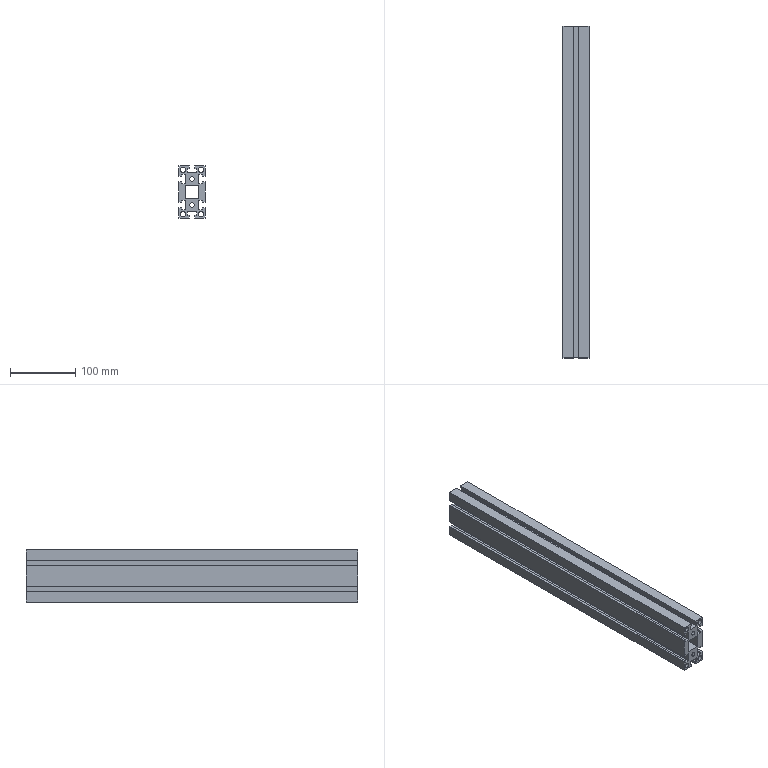Part | STEP file | 1 solid | 86 faces | box 40 x 510 x 80 mm | volume 928333 mm3 | plane 58 | cylinder 20 | cone 8 | commonest cylinder face diameters 6.8 x8 8 x8 6.7 x4